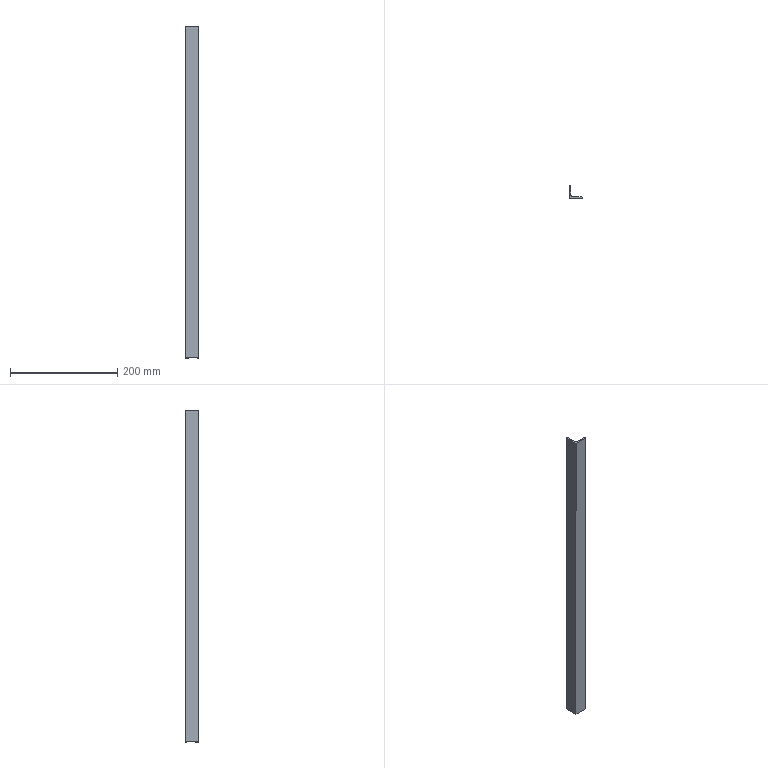Part | SolidWorks | features BaseBody 1 | 1 solid | 9 faces | box 25 x 25 x 620 mm | volume 86223 mm3 | plane 6 | cylinder 3 | commonest cylinder face diameters 6 x3
STEP:
#1=CARTESIAN_POINT('',(3.,22.,310.));
#2=VERTEX_POINT('',#1);
#3=CARTESIAN_POINT('',(0.,25.,310.));
#4=VERTEX_POINT('',#3);
#5=CARTESIAN_POINT('',(0.,22.,310.));
#6=DIRECTION('',(0.,0.,1.));
#7=DIRECTION('',(-1.,0.,0.));
#8=AXIS2_PLACEMENT_3D('',#5,#6,#7);
#9=CIRCLE('',#8,3.);
#10=EDGE_CURVE('',#2,#4,#9,.T.);
#11=ORIENTED_EDGE('',*,*,#10,.F.);
#12=CARTESIAN_POINT('',(3.,22.,-310.));
#13=VERTEX_POINT('',#12);
#14=CARTESIAN_POINT('',(3.,22.,310.));
#15=DIRECTION('',(0.,0.,1.));
#16=VECTOR('',#15,1000.);
#17=LINE('',#14,#16);
#18=EDGE_CURVE('',#13,#2,#17,.T.);
#19=ORIENTED_EDGE('',*,*,#18,.F.);
#20=CARTESIAN_POINT('',(0.,25.,-310.));
#21=VERTEX_POINT('',#20);
#22=CARTESIAN_POINT('',(0.,22.,-310.));
#23=DIRECTION('',(0.,0.,-1.));
#24=DIRECTION('',(-1.,0.,0.));
#25=AXIS2_PLACEMENT_3D('',#22,#23,#24);
#26=CIRCLE('',#25,3.);
#27=EDGE_CURVE('',#21,#13,#26,.T.);
#28=ORIENTED_EDGE('',*,*,#27,.F.);
#29=CARTESIAN_POINT('',(0.,25.,310.));
#30=DIRECTION('',(0.,0.,-1.));
#31=VECTOR('',#30,1000.);
#32=LINE('',#29,#31);
#33=EDGE_CURVE('',#4,#21,#32,.T.);
#34=ORIENTED_EDGE('',*,*,#33,.F.);
#35=EDGE_LOOP('',(#11,#19,#28,#34));
#36=FACE_OUTER_BOUND('',#35,.T.);
#37=CARTESIAN_POINT('',(0.,22.,310.));
#38=DIRECTION('',(0.,0.,-1.));
#39=DIRECTION('',(-1.,0.,0.));
#40=AXIS2_PLACEMENT_3D('',#37,#38,#39);
#41=CYLINDRICAL_SURFACE('',#40,3.);
#42=ADVANCED_FACE('',(#36),#41,.T.);
#43=CARTESIAN_POINT('',(25.,0.,310.));
#44=VERTEX_POINT('',#43);
#45=CARTESIAN_POINT('',(22.,3.,310.));
#46=VERTEX_POINT('',#45);
#47=CARTESIAN_POINT('',(22.,0.,310.));
#48=DIRECTION('',(0.,0.,1.));
#49=DIRECTION('',(-1.,0.,0.));
#50=AXIS2_PLACEMENT_3D('',#47,#48,#49);
#51=CIRCLE('',#50,3.);
#52=EDGE_CURVE('',#44,#46,#51,.T.);
#53=ORIENTED_EDGE('',*,*,#52,.F.);
#54=CARTESIAN_POINT('',(25.,0.,-310.));
#55=VERTEX_POINT('',#54);
#56=CARTESIAN_POINT('',(25.,0.,310.));
#57=DIRECTION('',(0.,0.,-1.));
#58=VECTOR('',#57,1000.);
#59=LINE('',#56,#58);
#60=EDGE_CURVE('',#44,#55,#59,.T.);
#61=ORIENTED_EDGE('',*,*,#60,.T.);
#62=CARTESIAN_POINT('',(22.,3.,-310.));
#63=VERTEX_POINT('',#62);
#64=CARTESIAN_POINT('',(22.,0.,-310.));
#65=DIRECTION('',(0.,0.,-1.));
#66=DIRECTION('',(-1.,0.,0.));
#67=AXIS2_PLACEMENT_3D('',#64,#65,#66);
#68=CIRCLE('',#67,3.);
#69=EDGE_CURVE('',#63,#55,#68,.T.);
#70=ORIENTED_EDGE('',*,*,#69,.F.);
#71=CARTESIAN_POINT('',(22.,3.,310.));
#72=DIRECTION('',(0.,0.,-1.));
#73=VECTOR('',#72,1000.);
#74=LINE('',#71,#73);
#75=EDGE_CURVE('',#46,#63,#74,.T.);
#76=ORIENTED_EDGE('',*,*,#75,.F.);
#77=EDGE_LOOP('',(#53,#61,#70,#76));
#78=FACE_OUTER_BOUND('',#77,.T.);
#79=CARTESIAN_POINT('',(22.,0.,310.));
#80=DIRECTION('',(0.,0.,-1.));
#81=DIRECTION('',(-1.,0.,0.));
#82=AXIS2_PLACEMENT_3D('',#79,#80,#81);
#83=CYLINDRICAL_SURFACE('',#82,3.);
#84=ADVANCED_FACE('',(#78),#83,.T.);
#85=CARTESIAN_POINT('',(6.,3.,310.));
#86=VERTEX_POINT('',#85);
#87=CARTESIAN_POINT('',(3.,6.,310.));
#88=VERTEX_POINT('',#87);
#89=CARTESIAN_POINT('',(6.,6.,310.));
#90=DIRECTION('',(0.,0.,-1.));
#91=DIRECTION('',(-1.,0.,0.));
#92=AXIS2_PLACEMENT_3D('',#89,#90,#91);
#93=CIRCLE('',#92,3.);
#94=EDGE_CURVE('',#86,#88,#93,.T.);
#95=ORIENTED_EDGE('',*,*,#94,.F.);
#96=CARTESIAN_POINT('',(6.,3.,-310.));
#97=VERTEX_POINT('',#96);
#98=CARTESIAN_POINT('',(6.,3.,310.));
#99=DIRECTION('',(0.,0.,1.));
#100=VECTOR('',#99,1000.);
#101=LINE('',#98,#100);
#102=EDGE_CURVE('',#97,#86,#101,.T.);
#103=ORIENTED_EDGE('',*,*,#102,.F.);
#104=CARTESIAN_POINT('',(3.,6.,-310.));
#105=VERTEX_POINT('',#104);
#106=CARTESIAN_POINT('',(6.,6.,-310.));
#107=DIRECTION('',(0.,0.,1.));
#108=DIRECTION('',(-1.,0.,0.));
#109=AXIS2_PLACEMENT_3D('',#106,#107,#108);
#110=CIRCLE('',#109,3.);
#111=EDGE_CURVE('',#105,#97,#110,.T.);
#112=ORIENTED_EDGE('',*,*,#111,.F.);
#113=CARTESIAN_POINT('',(3.,6.,-310.));
#114=DIRECTION('',(0.,0.,-1.));
#115=VECTOR('',#114,1000.);
#116=LINE('',#113,#115);
#117=EDGE_CURVE('',#88,#105,#116,.T.);
#118=ORIENTED_EDGE('',*,*,#117,.F.);
#119=EDGE_LOOP('',(#95,#103,#112,#118));
#120=FACE_OUTER_BOUND('',#119,.T.);
#121=CARTESIAN_POINT('',(6.,6.,310.));
#122=DIRECTION('',(0.,0.,1.));
#123=DIRECTION('',(1.,0.,0.));
#124=AXIS2_PLACEMENT_3D('',#121,#122,#123);
#125=CYLINDRICAL_SURFACE('',#124,3.);
#126=ADVANCED_FACE('',(#120),#125,.F.);
#127=CARTESIAN_POINT('',(3.,3.,-310.));
#128=DIRECTION('',(-1.,0.,0.));
#129=VECTOR('',#128,1000.);
#130=LINE('',#127,#129);
#131=EDGE_CURVE('',#63,#97,#130,.T.);
#132=ORIENTED_EDGE('',*,*,#131,.F.);
#133=ORIENTED_EDGE('',*,*,#69,.T.);
#134=CARTESIAN_POINT('',(0.,0.,-310.));
#135=VERTEX_POINT('',#134);
#136=CARTESIAN_POINT('',(0.,0.,-310.));
#137=DIRECTION('',(1.,0.,0.));
#138=VECTOR('',#137,1000.);
#139=LINE('',#136,#138);
#140=EDGE_CURVE('',#135,#55,#139,.T.);
#141=ORIENTED_EDGE('',*,*,#140,.F.);
#142=CARTESIAN_POINT('',(0.,0.,-310.));
#143=DIRECTION('',(0.,-1.,0.));
#144=VECTOR('',#143,1000.);
#145=LINE('',#142,#144);
#146=EDGE_CURVE('',#21,#135,#145,.T.);
#147=ORIENTED_EDGE('',*,*,#146,.F.);
#148=ORIENTED_EDGE('',*,*,#27,.T.);
#149=CARTESIAN_POINT('',(3.,25.,-310.));
#150=DIRECTION('',(0.,1.,0.));
#151=VECTOR('',#150,1000.);
#152=LINE('',#149,#151);
#153=EDGE_CURVE('',#105,#13,#152,.T.);
#154=ORIENTED_EDGE('',*,*,#153,.F.);
#155=ORIENTED_EDGE('',*,*,#111,.T.);
#156=EDGE_LOOP('',(#132,#133,#141,#147,#148,#154,#155));
#157=FACE_OUTER_BOUND('',#156,.T.);
#158=CARTESIAN_POINT('',(0.,0.,-310.));
#159=DIRECTION('',(0.,0.,-1.));
#160=DIRECTION('',(0.,-1.,0.));
#161=AXIS2_PLACEMENT_3D('',#158,#159,#160);
#162=PLANE('',#161);
#163=ADVANCED_FACE('',(#157),#162,.T.);
#164=CARTESIAN_POINT('',(0.,0.,310.));
#165=VERTEX_POINT('',#164);
#166=CARTESIAN_POINT('',(0.,0.,310.));
#167=DIRECTION('',(1.,0.,0.));
#168=VECTOR('',#167,1000.);
#169=LINE('',#166,#168);
#170=EDGE_CURVE('',#165,#44,#169,.T.);
#171=ORIENTED_EDGE('',*,*,#170,.T.);
#172=ORIENTED_EDGE('',*,*,#52,.T.);
#173=CARTESIAN_POINT('',(3.,3.,310.));
#174=DIRECTION('',(-1.,0.,0.));
#175=VECTOR('',#174,1000.);
#176=LINE('',#173,#175);
#177=EDGE_CURVE('',#46,#86,#176,.T.);
#178=ORIENTED_EDGE('',*,*,#177,.T.);
#179=ORIENTED_EDGE('',*,*,#94,.T.);
#180=CARTESIAN_POINT('',(3.,25.,310.));
#181=DIRECTION('',(0.,1.,0.));
#182=VECTOR('',#181,1000.);
#183=LINE('',#180,#182);
#184=EDGE_CURVE('',#88,#2,#183,.T.);
#185=ORIENTED_EDGE('',*,*,#184,.T.);
#186=ORIENTED_EDGE('',*,*,#10,.T.);
#187=CARTESIAN_POINT('',(0.,0.,310.));
#188=DIRECTION('',(0.,-1.,0.));
#189=VECTOR('',#188,1000.);
#190=LINE('',#187,#189);
#191=EDGE_CURVE('',#4,#165,#190,.T.);
#192=ORIENTED_EDGE('',*,*,#191,.T.);
#193=EDGE_LOOP('',(#171,#172,#178,#179,#185,#186,#192));
#194=FACE_OUTER_BOUND('',#193,.T.);
#195=CARTESIAN_POINT('',(0.,0.,310.));
#196=DIRECTION('',(0.,0.,-1.));
#197=DIRECTION('',(0.,-1.,0.));
#198=AXIS2_PLACEMENT_3D('',#195,#196,#197);
#199=PLANE('',#198);
#200=ADVANCED_FACE('',(#194),#199,.F.);
#201=ORIENTED_EDGE('',*,*,#153,.T.);
#202=ORIENTED_EDGE('',*,*,#18,.T.);
#203=ORIENTED_EDGE('',*,*,#184,.F.);
#204=ORIENTED_EDGE('',*,*,#117,.T.);
#205=EDGE_LOOP('',(#201,#202,#203,#204));
#206=FACE_OUTER_BOUND('',#205,.T.);
#207=CARTESIAN_POINT('',(3.,25.,310.));
#208=DIRECTION('',(-1.,0.,0.));
#209=DIRECTION('',(0.,1.,0.));
#210=AXIS2_PLACEMENT_3D('',#207,#208,#209);
#211=PLANE('',#210);
#212=ADVANCED_FACE('',(#206),#211,.F.);
#213=ORIENTED_EDGE('',*,*,#177,.F.);
#214=ORIENTED_EDGE('',*,*,#75,.T.);
#215=ORIENTED_EDGE('',*,*,#131,.T.);
#216=ORIENTED_EDGE('',*,*,#102,.T.);
#217=EDGE_LOOP('',(#213,#214,#215,#216));
#218=FACE_OUTER_BOUND('',#217,.T.);
#219=CARTESIAN_POINT('',(3.,3.,310.));
#220=DIRECTION('',(0.,-1.,0.));
#221=DIRECTION('',(0.,0.,-1.));
#222=AXIS2_PLACEMENT_3D('',#219,#220,#221);
#223=PLANE('',#222);
#224=ADVANCED_FACE('',(#218),#223,.F.);
#225=ORIENTED_EDGE('',*,*,#140,.T.);
#226=ORIENTED_EDGE('',*,*,#60,.F.);
#227=ORIENTED_EDGE('',*,*,#170,.F.);
#228=CARTESIAN_POINT('',(0.,0.,310.));
#229=DIRECTION('',(0.,0.,-1.));
#230=VECTOR('',#229,1000.);
#231=LINE('',#228,#230);
#232=EDGE_CURVE('',#165,#135,#231,.T.);
#233=ORIENTED_EDGE('',*,*,#232,.T.);
#234=EDGE_LOOP('',(#225,#226,#227,#233));
#235=FACE_OUTER_BOUND('',#234,.T.);
#236=CARTESIAN_POINT('',(0.,0.,310.));
#237=DIRECTION('',(0.,1.,0.));
#238=DIRECTION('',(1.,0.,0.));
#239=AXIS2_PLACEMENT_3D('',#236,#237,#238);
#240=PLANE('',#239);
#241=ADVANCED_FACE('',(#235),#240,.F.);
#242=ORIENTED_EDGE('',*,*,#146,.T.);
#243=ORIENTED_EDGE('',*,*,#232,.F.);
#244=ORIENTED_EDGE('',*,*,#191,.F.);
#245=ORIENTED_EDGE('',*,*,#33,.T.);
#246=EDGE_LOOP('',(#242,#243,#244,#245));
#247=FACE_OUTER_BOUND('',#246,.T.);
#248=CARTESIAN_POINT('',(0.,0.,310.));
#249=DIRECTION('',(1.,0.,0.));
#250=DIRECTION('',(0.,1.,0.));
#251=AXIS2_PLACEMENT_3D('',#248,#249,#250);
#252=PLANE('',#251);
#253=ADVANCED_FACE('',(#247),#252,.F.);
#254=CLOSED_SHELL('',(#42,#84,#126,#163,#200,#212,#224,#241,#253));
#255=MANIFOLD_SOLID_BREP('',#254);
#256=CARTESIAN_POINT('',(0.,0.,0.));
#257=DIRECTION('',(0.,0.,1.));
#258=DIRECTION('',(1.,0.,0.));
#259=AXIS2_PLACEMENT_3D('',#256,#257,#258);
#260=(LENGTH_UNIT()NAMED_UNIT(*)SI_UNIT(.MILLI.,.METRE.));
#261=UNCERTAINTY_MEASURE_WITH_UNIT(LENGTH_MEASURE(0.00001),#260,'','');
#262=(NAMED_UNIT(*)PLANE_ANGLE_UNIT()SI_UNIT($,.RADIAN.));
#263=(NAMED_UNIT(*)SI_UNIT($,.STERADIAN.)SOLID_ANGLE_UNIT());
#264=(GEOMETRIC_REPRESENTATION_CONTEXT(3)GLOBAL_UNCERTAINTY_ASSIGNED_CONTEXT((#261))GLOBAL_UNIT_ASSIGNED_CONTEXT((#260,#262,#263))REPRESENTATION_CONTEXT('',''));
#265=ADVANCED_BREP_SHAPE_REPRESENTATION('',(#255,#259),#264);